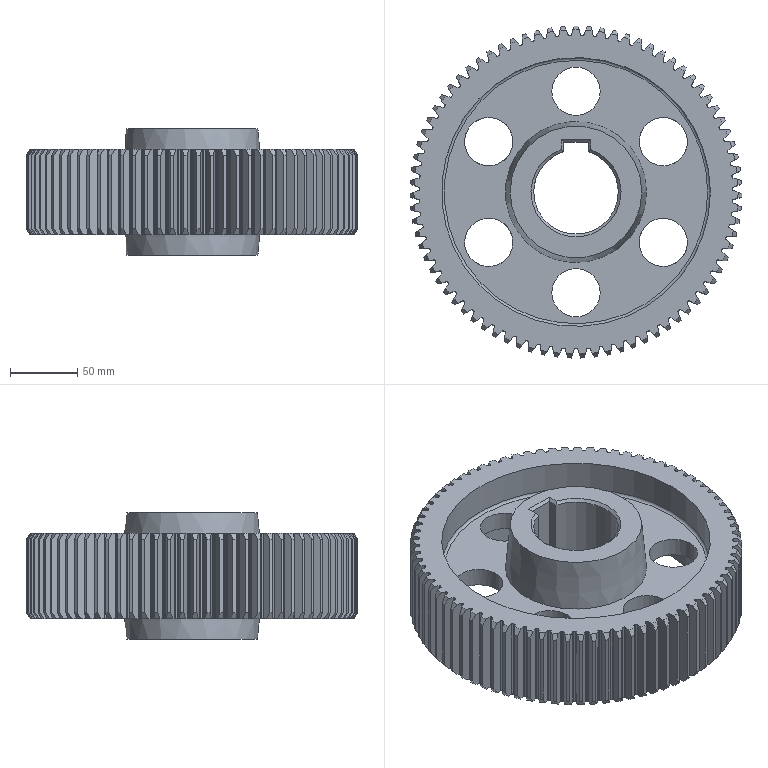Part | NX | features BREP 79, META 79, DATUM_CSYS 10, SKETCH 9, EXTRUDE 8, BLEND 1, CHAMFER 1, CPROJ 1, CYLINDER 1, FSET 1, SWP104 1 | 1 solid | 662 faces | box 247.038 x 246.995 x 94 mm | volume 1592670 mm3 | spline 395 | cone 162 | cylinder 88 | plane 15 | torus 2 | commonest cylinder face diameters 233.325 x79 36 x6 200 x2 63 x1